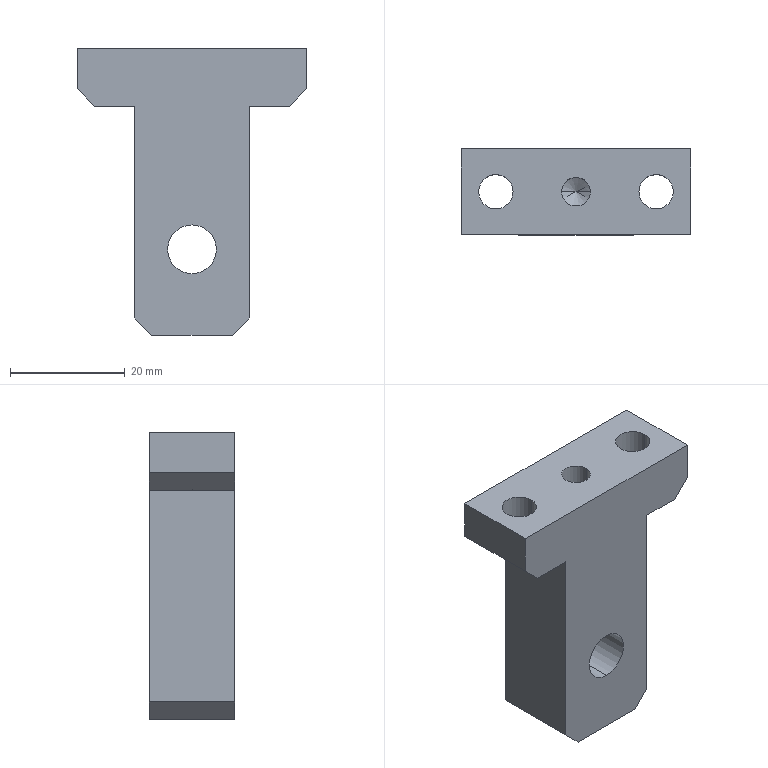Part | STEP file | PN_0028_default | 1 solid | 24 faces | box 40 x 15 x 50 mm | volume 16009 mm3 | plane 14 | cylinder 8 | cone 2 | commonest cylinder face diameters 6 x4 5 x2 8.5 x2